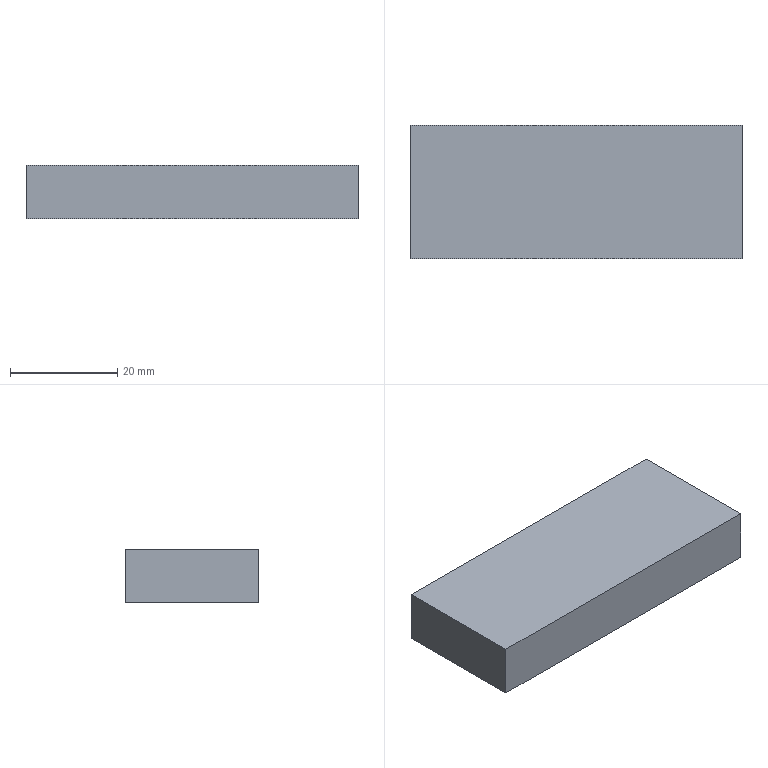Part | STEP file | 001-010-Waste cylinder adapter plate | 1 solid | 6 faces | box 62 x 25 x 10 mm | volume 15500 mm3 | plane 6
STEP:
#1=CARTESIAN_POINT('',(0.,0.,0.));
#2=DIRECTION('',(0.,0.,1.));
#3=DIRECTION('',(1.,0.,0.));
#4=AXIS2_PLACEMENT_3D('',#1,#2,#3);
#5=CARTESIAN_POINT('',(31.,-12.5,0.));
#6=VERTEX_POINT('',#5);
#7=CARTESIAN_POINT('',(31.,12.5,0.));
#8=VERTEX_POINT('',#7);
#9=CARTESIAN_POINT('',(31.,-12.5,0.));
#10=DIRECTION('',(0.,1.,0.));
#11=VECTOR('',#10,1.);
#12=LINE('',#9,#11);
#13=CARTESIAN_POINT('',(31.,-12.5,10.));
#14=DIRECTION('',(-1.,0.,0.));
#15=DIRECTION('',(0.,0.,1.));
#16=AXIS2_PLACEMENT_3D('',#13,#14,#15);
#17=PLANE('',#16);
#18=CARTESIAN_POINT('',(-10.,0.));
#19=DIRECTION('',(0.,1.));
#20=VECTOR('',#19,1.);
#21=LINE('',#18,#20);
#22=(GEOMETRIC_REPRESENTATION_CONTEXT(2)PARAMETRIC_REPRESENTATION_CONTEXT()REPRESENTATION_CONTEXT('',''));
#23=DEFINITIONAL_REPRESENTATION('',(#21),#22);
#24=PCURVE('',#17,#23);
#25=CARTESIAN_POINT('',(0.,0.,0.));
#26=DIRECTION('',(0.,0.,-1.));
#27=DIRECTION('',(-1.,0.,0.));
#28=AXIS2_PLACEMENT_3D('',#25,#26,#27);
#29=PLANE('',#28);
#30=CARTESIAN_POINT('',(-31.,-12.5));
#31=DIRECTION('',(0.,1.));
#32=VECTOR('',#31,1.);
#33=LINE('',#30,#32);
#34=(GEOMETRIC_REPRESENTATION_CONTEXT(2)PARAMETRIC_REPRESENTATION_CONTEXT()REPRESENTATION_CONTEXT('',''));
#35=DEFINITIONAL_REPRESENTATION('',(#33),#34);
#36=PCURVE('',#29,#35);
#37=SURFACE_CURVE('',#12,(#24,#36),.PCURVE_S1.);
#38=EDGE_CURVE('',#6,#8,#37,.T.);
#39=ORIENTED_EDGE('',*,*,#38,.T.);
#40=CARTESIAN_POINT('',(31.,12.5,10.));
#41=VERTEX_POINT('',#40);
#42=CARTESIAN_POINT('',(31.,12.5,10.));
#43=DIRECTION('',(0.,0.,-1.));
#44=VECTOR('',#43,1.);
#45=LINE('',#42,#44);
#46=CARTESIAN_POINT('',(0.,25.));
#47=DIRECTION('',(-1.,0.));
#48=VECTOR('',#47,1.);
#49=LINE('',#46,#48);
#50=(GEOMETRIC_REPRESENTATION_CONTEXT(2)PARAMETRIC_REPRESENTATION_CONTEXT()REPRESENTATION_CONTEXT('',''));
#51=DEFINITIONAL_REPRESENTATION('',(#49),#50);
#52=PCURVE('',#17,#51);
#53=CARTESIAN_POINT('',(-31.,12.5,10.));
#54=DIRECTION('',(0.,-1.,0.));
#55=DIRECTION('',(0.,0.,-1.));
#56=AXIS2_PLACEMENT_3D('',#53,#54,#55);
#57=PLANE('',#56);
#58=CARTESIAN_POINT('',(0.,62.));
#59=DIRECTION('',(1.,0.));
#60=VECTOR('',#59,1.);
#61=LINE('',#58,#60);
#62=(GEOMETRIC_REPRESENTATION_CONTEXT(2)PARAMETRIC_REPRESENTATION_CONTEXT()REPRESENTATION_CONTEXT('',''));
#63=DEFINITIONAL_REPRESENTATION('',(#61),#62);
#64=PCURVE('',#57,#63);
#65=SURFACE_CURVE('',#45,(#52,#64),.PCURVE_S1.);
#66=EDGE_CURVE('',#41,#8,#65,.T.);
#67=ORIENTED_EDGE('',*,*,#66,.F.);
#68=CARTESIAN_POINT('',(31.,-12.5,10.));
#69=VERTEX_POINT('',#68);
#70=CARTESIAN_POINT('',(31.,-12.5,10.));
#71=DIRECTION('',(0.,1.,0.));
#72=VECTOR('',#71,1.);
#73=LINE('',#70,#72);
#74=CARTESIAN_POINT('',(0.,0.));
#75=DIRECTION('',(0.,1.));
#76=VECTOR('',#75,1.);
#77=LINE('',#74,#76);
#78=(GEOMETRIC_REPRESENTATION_CONTEXT(2)PARAMETRIC_REPRESENTATION_CONTEXT()REPRESENTATION_CONTEXT('',''));
#79=DEFINITIONAL_REPRESENTATION('',(#77),#78);
#80=PCURVE('',#17,#79);
#81=CARTESIAN_POINT('',(0.,0.,10.));
#82=DIRECTION('',(0.,0.,-1.));
#83=DIRECTION('',(-1.,0.,0.));
#84=AXIS2_PLACEMENT_3D('',#81,#82,#83);
#85=PLANE('',#84);
#86=CARTESIAN_POINT('',(-31.,-12.5));
#87=DIRECTION('',(0.,1.));
#88=VECTOR('',#87,1.);
#89=LINE('',#86,#88);
#90=(GEOMETRIC_REPRESENTATION_CONTEXT(2)PARAMETRIC_REPRESENTATION_CONTEXT()REPRESENTATION_CONTEXT('',''));
#91=DEFINITIONAL_REPRESENTATION('',(#89),#90);
#92=PCURVE('',#85,#91);
#93=SURFACE_CURVE('',#73,(#80,#92),.PCURVE_S1.);
#94=EDGE_CURVE('',#69,#41,#93,.T.);
#95=ORIENTED_EDGE('',*,*,#94,.F.);
#96=CARTESIAN_POINT('',(31.,-12.5,10.));
#97=DIRECTION('',(0.,0.,-1.));
#98=VECTOR('',#97,1.);
#99=LINE('',#96,#98);
#100=CARTESIAN_POINT('',(0.,0.));
#101=DIRECTION('',(-1.,0.));
#102=VECTOR('',#101,1.);
#103=LINE('',#100,#102);
#104=(GEOMETRIC_REPRESENTATION_CONTEXT(2)PARAMETRIC_REPRESENTATION_CONTEXT()REPRESENTATION_CONTEXT('',''));
#105=DEFINITIONAL_REPRESENTATION('',(#103),#104);
#106=PCURVE('',#17,#105);
#107=CARTESIAN_POINT('',(-31.,-12.5,10.));
#108=DIRECTION('',(0.,1.,0.));
#109=DIRECTION('',(0.,0.,1.));
#110=AXIS2_PLACEMENT_3D('',#107,#108,#109);
#111=PLANE('',#110);
#112=CARTESIAN_POINT('',(0.,62.));
#113=DIRECTION('',(-1.,0.));
#114=VECTOR('',#113,1.);
#115=LINE('',#112,#114);
#116=(GEOMETRIC_REPRESENTATION_CONTEXT(2)PARAMETRIC_REPRESENTATION_CONTEXT()REPRESENTATION_CONTEXT('',''));
#117=DEFINITIONAL_REPRESENTATION('',(#115),#116);
#118=PCURVE('',#111,#117);
#119=SURFACE_CURVE('',#99,(#106,#118),.PCURVE_S1.);
#120=EDGE_CURVE('',#69,#6,#119,.T.);
#121=ORIENTED_EDGE('',*,*,#120,.T.);
#122=EDGE_LOOP('',(#39,#67,#95,#121));
#123=FACE_BOUND('',#122,.T.);
#124=ADVANCED_FACE('',(#123),#17,.F.);
#125=CARTESIAN_POINT('',(-31.,12.5,0.));
#126=VERTEX_POINT('',#125);
#127=CARTESIAN_POINT('',(-31.,12.5,0.));
#128=DIRECTION('',(-1.,0.,0.));
#129=VECTOR('',#128,1.);
#130=LINE('',#127,#129);
#131=CARTESIAN_POINT('',(10.,0.));
#132=DIRECTION('',(0.,-1.));
#133=VECTOR('',#132,1.);
#134=LINE('',#131,#133);
#135=(GEOMETRIC_REPRESENTATION_CONTEXT(2)PARAMETRIC_REPRESENTATION_CONTEXT()REPRESENTATION_CONTEXT('',''));
#136=DEFINITIONAL_REPRESENTATION('',(#134),#135);
#137=PCURVE('',#57,#136);
#138=CARTESIAN_POINT('',(31.,12.5));
#139=DIRECTION('',(1.,0.));
#140=VECTOR('',#139,1.);
#141=LINE('',#138,#140);
#142=(GEOMETRIC_REPRESENTATION_CONTEXT(2)PARAMETRIC_REPRESENTATION_CONTEXT()REPRESENTATION_CONTEXT('',''));
#143=DEFINITIONAL_REPRESENTATION('',(#141),#142);
#144=PCURVE('',#29,#143);
#145=SURFACE_CURVE('',#130,(#137,#144),.PCURVE_S1.);
#146=EDGE_CURVE('',#8,#126,#145,.T.);
#147=ORIENTED_EDGE('',*,*,#146,.T.);
#148=CARTESIAN_POINT('',(-31.,12.5,10.));
#149=VERTEX_POINT('',#148);
#150=CARTESIAN_POINT('',(-31.,12.5,10.));
#151=DIRECTION('',(0.,0.,-1.));
#152=VECTOR('',#151,1.);
#153=LINE('',#150,#152);
#154=CARTESIAN_POINT('',(0.,0.));
#155=DIRECTION('',(1.,0.));
#156=VECTOR('',#155,1.);
#157=LINE('',#154,#156);
#158=(GEOMETRIC_REPRESENTATION_CONTEXT(2)PARAMETRIC_REPRESENTATION_CONTEXT()REPRESENTATION_CONTEXT('',''));
#159=DEFINITIONAL_REPRESENTATION('',(#157),#158);
#160=PCURVE('',#57,#159);
#161=CARTESIAN_POINT('',(-31.,-12.5,10.));
#162=DIRECTION('',(1.,0.,0.));
#163=DIRECTION('',(0.,0.,-1.));
#164=AXIS2_PLACEMENT_3D('',#161,#162,#163);
#165=PLANE('',#164);
#166=CARTESIAN_POINT('',(0.,25.));
#167=DIRECTION('',(1.,0.));
#168=VECTOR('',#167,1.);
#169=LINE('',#166,#168);
#170=(GEOMETRIC_REPRESENTATION_CONTEXT(2)PARAMETRIC_REPRESENTATION_CONTEXT()REPRESENTATION_CONTEXT('',''));
#171=DEFINITIONAL_REPRESENTATION('',(#169),#170);
#172=PCURVE('',#165,#171);
#173=SURFACE_CURVE('',#153,(#160,#172),.PCURVE_S1.);
#174=EDGE_CURVE('',#149,#126,#173,.T.);
#175=ORIENTED_EDGE('',*,*,#174,.F.);
#176=CARTESIAN_POINT('',(-31.,12.5,10.));
#177=DIRECTION('',(-1.,0.,0.));
#178=VECTOR('',#177,1.);
#179=LINE('',#176,#178);
#180=CARTESIAN_POINT('',(0.,0.));
#181=DIRECTION('',(0.,-1.));
#182=VECTOR('',#181,1.);
#183=LINE('',#180,#182);
#184=(GEOMETRIC_REPRESENTATION_CONTEXT(2)PARAMETRIC_REPRESENTATION_CONTEXT()REPRESENTATION_CONTEXT('',''));
#185=DEFINITIONAL_REPRESENTATION('',(#183),#184);
#186=PCURVE('',#57,#185);
#187=CARTESIAN_POINT('',(31.,12.5));
#188=DIRECTION('',(1.,0.));
#189=VECTOR('',#188,1.);
#190=LINE('',#187,#189);
#191=(GEOMETRIC_REPRESENTATION_CONTEXT(2)PARAMETRIC_REPRESENTATION_CONTEXT()REPRESENTATION_CONTEXT('',''));
#192=DEFINITIONAL_REPRESENTATION('',(#190),#191);
#193=PCURVE('',#85,#192);
#194=SURFACE_CURVE('',#179,(#186,#193),.PCURVE_S1.);
#195=EDGE_CURVE('',#41,#149,#194,.T.);
#196=ORIENTED_EDGE('',*,*,#195,.F.);
#197=ORIENTED_EDGE('',*,*,#66,.T.);
#198=EDGE_LOOP('',(#147,#175,#196,#197));
#199=FACE_BOUND('',#198,.T.);
#200=ADVANCED_FACE('',(#199),#57,.F.);
#201=CARTESIAN_POINT('',(-31.,-12.5,0.));
#202=VERTEX_POINT('',#201);
#203=CARTESIAN_POINT('',(-31.,-12.5,0.));
#204=DIRECTION('',(0.,-1.,0.));
#205=VECTOR('',#204,1.);
#206=LINE('',#203,#205);
#207=CARTESIAN_POINT('',(10.,0.));
#208=DIRECTION('',(0.,-1.));
#209=VECTOR('',#208,1.);
#210=LINE('',#207,#209);
#211=(GEOMETRIC_REPRESENTATION_CONTEXT(2)PARAMETRIC_REPRESENTATION_CONTEXT()REPRESENTATION_CONTEXT('',''));
#212=DEFINITIONAL_REPRESENTATION('',(#210),#211);
#213=PCURVE('',#165,#212);
#214=CARTESIAN_POINT('',(31.,-12.5));
#215=DIRECTION('',(0.,-1.));
#216=VECTOR('',#215,1.);
#217=LINE('',#214,#216);
#218=(GEOMETRIC_REPRESENTATION_CONTEXT(2)PARAMETRIC_REPRESENTATION_CONTEXT()REPRESENTATION_CONTEXT('',''));
#219=DEFINITIONAL_REPRESENTATION('',(#217),#218);
#220=PCURVE('',#29,#219);
#221=SURFACE_CURVE('',#206,(#213,#220),.PCURVE_S1.);
#222=EDGE_CURVE('',#126,#202,#221,.T.);
#223=ORIENTED_EDGE('',*,*,#222,.T.);
#224=CARTESIAN_POINT('',(-31.,-12.5,10.));
#225=VERTEX_POINT('',#224);
#226=CARTESIAN_POINT('',(-31.,-12.5,10.));
#227=DIRECTION('',(0.,0.,-1.));
#228=VECTOR('',#227,1.);
#229=LINE('',#226,#228);
#230=CARTESIAN_POINT('',(0.,0.));
#231=DIRECTION('',(1.,0.));
#232=VECTOR('',#231,1.);
#233=LINE('',#230,#232);
#234=(GEOMETRIC_REPRESENTATION_CONTEXT(2)PARAMETRIC_REPRESENTATION_CONTEXT()REPRESENTATION_CONTEXT('',''));
#235=DEFINITIONAL_REPRESENTATION('',(#233),#234);
#236=PCURVE('',#165,#235);
#237=CARTESIAN_POINT('',(0.,0.));
#238=DIRECTION('',(-1.,0.));
#239=VECTOR('',#238,1.);
#240=LINE('',#237,#239);
#241=(GEOMETRIC_REPRESENTATION_CONTEXT(2)PARAMETRIC_REPRESENTATION_CONTEXT()REPRESENTATION_CONTEXT('',''));
#242=DEFINITIONAL_REPRESENTATION('',(#240),#241);
#243=PCURVE('',#111,#242);
#244=SURFACE_CURVE('',#229,(#236,#243),.PCURVE_S1.);
#245=EDGE_CURVE('',#225,#202,#244,.T.);
#246=ORIENTED_EDGE('',*,*,#245,.F.);
#247=CARTESIAN_POINT('',(-31.,-12.5,10.));
#248=DIRECTION('',(0.,-1.,0.));
#249=VECTOR('',#248,1.);
#250=LINE('',#247,#249);
#251=CARTESIAN_POINT('',(0.,0.));
#252=DIRECTION('',(0.,-1.));
#253=VECTOR('',#252,1.);
#254=LINE('',#251,#253);
#255=(GEOMETRIC_REPRESENTATION_CONTEXT(2)PARAMETRIC_REPRESENTATION_CONTEXT()REPRESENTATION_CONTEXT('',''));
#256=DEFINITIONAL_REPRESENTATION('',(#254),#255);
#257=PCURVE('',#165,#256);
#258=CARTESIAN_POINT('',(31.,-12.5));
#259=DIRECTION('',(0.,-1.));
#260=VECTOR('',#259,1.);
#261=LINE('',#258,#260);
#262=(GEOMETRIC_REPRESENTATION_CONTEXT(2)PARAMETRIC_REPRESENTATION_CONTEXT()REPRESENTATION_CONTEXT('',''));
#263=DEFINITIONAL_REPRESENTATION('',(#261),#262);
#264=PCURVE('',#85,#263);
#265=SURFACE_CURVE('',#250,(#257,#264),.PCURVE_S1.);
#266=EDGE_CURVE('',#149,#225,#265,.T.);
#267=ORIENTED_EDGE('',*,*,#266,.F.);
#268=ORIENTED_EDGE('',*,*,#174,.T.);
#269=EDGE_LOOP('',(#223,#246,#267,#268));
#270=FACE_BOUND('',#269,.T.);
#271=ADVANCED_FACE('',(#270),#165,.F.);
#272=CARTESIAN_POINT('',(-31.,-12.5,0.));
#273=DIRECTION('',(1.,0.,0.));
#274=VECTOR('',#273,1.);
#275=LINE('',#272,#274);
#276=CARTESIAN_POINT('',(-10.,0.));
#277=DIRECTION('',(0.,1.));
#278=VECTOR('',#277,1.);
#279=LINE('',#276,#278);
#280=(GEOMETRIC_REPRESENTATION_CONTEXT(2)PARAMETRIC_REPRESENTATION_CONTEXT()REPRESENTATION_CONTEXT('',''));
#281=DEFINITIONAL_REPRESENTATION('',(#279),#280);
#282=PCURVE('',#111,#281);
#283=CARTESIAN_POINT('',(31.,-12.5));
#284=DIRECTION('',(-1.,0.));
#285=VECTOR('',#284,1.);
#286=LINE('',#283,#285);
#287=(GEOMETRIC_REPRESENTATION_CONTEXT(2)PARAMETRIC_REPRESENTATION_CONTEXT()REPRESENTATION_CONTEXT('',''));
#288=DEFINITIONAL_REPRESENTATION('',(#286),#287);
#289=PCURVE('',#29,#288);
#290=SURFACE_CURVE('',#275,(#282,#289),.PCURVE_S1.);
#291=EDGE_CURVE('',#202,#6,#290,.T.);
#292=ORIENTED_EDGE('',*,*,#291,.T.);
#293=ORIENTED_EDGE('',*,*,#120,.F.);
#294=CARTESIAN_POINT('',(-31.,-12.5,10.));
#295=DIRECTION('',(1.,0.,0.));
#296=VECTOR('',#295,1.);
#297=LINE('',#294,#296);
#298=CARTESIAN_POINT('',(0.,0.));
#299=DIRECTION('',(0.,1.));
#300=VECTOR('',#299,1.);
#301=LINE('',#298,#300);
#302=(GEOMETRIC_REPRESENTATION_CONTEXT(2)PARAMETRIC_REPRESENTATION_CONTEXT()REPRESENTATION_CONTEXT('',''));
#303=DEFINITIONAL_REPRESENTATION('',(#301),#302);
#304=PCURVE('',#111,#303);
#305=CARTESIAN_POINT('',(31.,-12.5));
#306=DIRECTION('',(-1.,0.));
#307=VECTOR('',#306,1.);
#308=LINE('',#305,#307);
#309=(GEOMETRIC_REPRESENTATION_CONTEXT(2)PARAMETRIC_REPRESENTATION_CONTEXT()REPRESENTATION_CONTEXT('',''));
#310=DEFINITIONAL_REPRESENTATION('',(#308),#309);
#311=PCURVE('',#85,#310);
#312=SURFACE_CURVE('',#297,(#304,#311),.PCURVE_S1.);
#313=EDGE_CURVE('',#225,#69,#312,.T.);
#314=ORIENTED_EDGE('',*,*,#313,.F.);
#315=ORIENTED_EDGE('',*,*,#245,.T.);
#316=EDGE_LOOP('',(#292,#293,#314,#315));
#317=FACE_BOUND('',#316,.T.);
#318=ADVANCED_FACE('',(#317),#111,.F.);
#319=ORIENTED_EDGE('',*,*,#94,.T.);
#320=ORIENTED_EDGE('',*,*,#195,.T.);
#321=ORIENTED_EDGE('',*,*,#266,.T.);
#322=ORIENTED_EDGE('',*,*,#313,.T.);
#323=EDGE_LOOP('',(#319,#320,#321,#322));
#324=FACE_BOUND('',#323,.T.);
#325=ADVANCED_FACE('',(#324),#85,.F.);
#326=ORIENTED_EDGE('',*,*,#38,.F.);
#327=ORIENTED_EDGE('',*,*,#291,.F.);
#328=ORIENTED_EDGE('',*,*,#222,.F.);
#329=ORIENTED_EDGE('',*,*,#146,.F.);
#330=EDGE_LOOP('',(#326,#327,#328,#329));
#331=FACE_BOUND('',#330,.T.);
#332=ADVANCED_FACE('',(#331),#29,.T.);
#333=CLOSED_SHELL('',(#124,#200,#271,#318,#325,#332));
#334=MANIFOLD_SOLID_BREP('',#333);
#335=(LENGTH_UNIT()NAMED_UNIT(*)SI_UNIT(.MILLI.,.METRE.));
#336=UNCERTAINTY_MEASURE_WITH_UNIT(LENGTH_MEASURE(0.0000001),#335,'','');
#337=(NAMED_UNIT(*)PLANE_ANGLE_UNIT()SI_UNIT($,.RADIAN.));
#338=(NAMED_UNIT(*)SI_UNIT($,.STERADIAN.)SOLID_ANGLE_UNIT());
#339=(GEOMETRIC_REPRESENTATION_CONTEXT(3)GLOBAL_UNCERTAINTY_ASSIGNED_CONTEXT((#336))GLOBAL_UNIT_ASSIGNED_CONTEXT((#335,#337,#338))REPRESENTATION_CONTEXT('',''));
#340=ADVANCED_BREP_SHAPE_REPRESENTATION('',(#4,#334),#339);